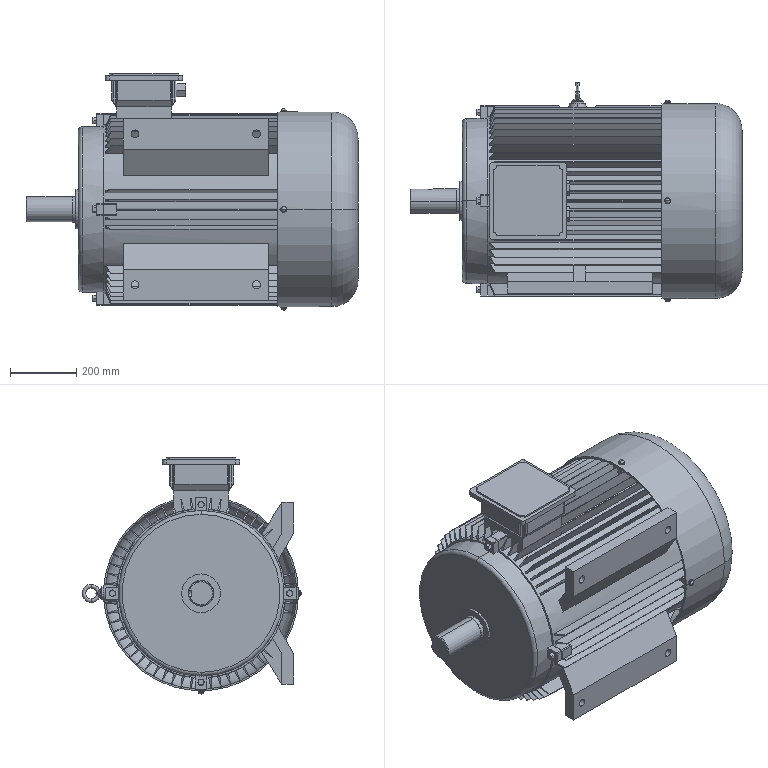Part | SolidWorks | features Boss 17, Cut 5, Revolution 5, Fillet 4, Chamfer 3, CirPattern 3, RevCut 2, 3DProfileFeature 1, LPattern 1, MirrorPattern 1, MoveCopyBody 1 | 2 solids | 614 faces | box 1005 x 665 x 715 mm | volume 186220759 mm3 | plane 377 | cone 138 | cylinder 79 | torus 12 | sphere 8 | commonest cylinder face diameters 16 x16 7.5 x12 18 x8 22.5 x8 24 x8 29.665 x4